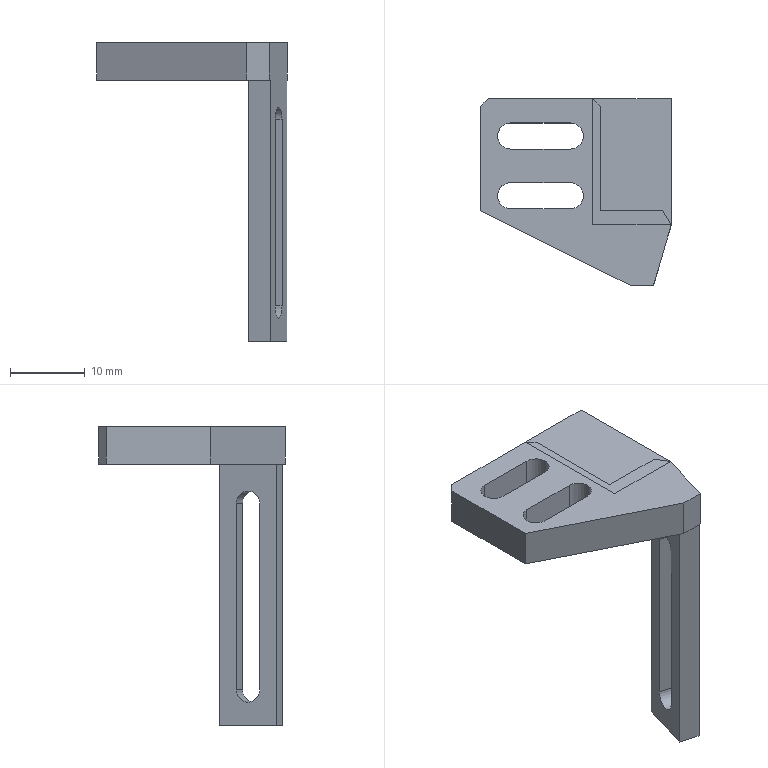NC program | NX | posted with a generic post | part box 25.523 x 25 x 40 mm
Whole program:
N10 G17 G21 G94 G90
(ZLEVEL_PROFILE_1_1 , TOOL : D4R0.5)
N12 T07 M6
N14 G54
N16 G17 G0 G90 X2.815 Y14.477 B0. C0. S7500 M3
N18 G43 Z30. H7
N20 Z0.948
N22 G94 G1 Z-0.052 F1000.
N24 X2.518 Y14.992
N26 G3 X2.172 Y15.192 R0.4
N28 G1 X-7.172 F2500.
N30 Y15.149 Z-0.078
N32 Y15.107 Z-0.105
N34 X-5. Y15.106
N36 X0.
N38 X2.172 Y15.107
N40 Y15.063 Z-0.131
N42 Y15.022 Z-0.157
N44 X0. Y15.021
N46 X-5.
N48 X-7.172 Y15.022
N50 Y14.978 Z-0.183
N52 Y14.936 Z-0.209
N54 X-5.
N56 X0.
N58 X2.172
N60 Y14.893 Z-0.235
N62 Y14.851 Z-0.261
N64 X0. Y14.85
N66 X-5.
N68 X-7.172 Y14.851
N70 Y14.808 Z-0.287
N72 Y14.766 Z-0.314
N74 X-5. Y14.765
N76 X0.
N78 X2.172 Y14.766
N80 Y14.722 Z-0.34
N82 Y14.68 Z-0.366
N84 X0.
N86 X-5.
N88 X-7.172
N90 Y14.637 Z-0.392
N92 Y14.595 Z-0.418
N94 X-5.
N96 X0.
N98 X2.172
N100 Y14.552 Z-0.444
N102 Y14.51 Z-0.47
N104 X0. Y14.509
N106 X-5.
N108 X-7.172 Y14.51
N110 Y14.467 Z-0.496
N112 Y14.425 Z-0.522
N114 X-5. Y14.424
N116 X0.
N118 X2.172 Y14.425
N120 Y14.381 Z-0.549
N122 Y14.339 Z-0.575
N124 X0.
N126 X-5.
N128 X-7.172
N130 Y14.296 Z-0.601
N132 Y14.254 Z-0.627
N134 X-5. Y14.253
N136 X0.
N138 X2.172 Y14.254
N140 Y14.211 Z-0.653
N142 Y14.169 Z-0.679
N144 X0. Y14.168
N146 X-5.
N148 X-7.172 Y14.169
N150 Y14.126 Z-0.705
N152 Y14.084 Z-0.731
N154 X-5. Y14.083
N156 X0.
N158 X2.172 Y14.084
N160 Y14.04 Z-0.758
N162 Y13.998 Z-0.784
N164 X0.
N166 X-5.
N168 X-7.172
N170 Y13.955 Z-0.81
N172 Y13.913 Z-0.836
N174 X-5. Y13.912
N176 X0.
N178 X2.172 Y13.913
N180 Y13.87 Z-0.862
N182 Y13.828 Z-0.888
N184 X0. Y13.827
N186 X-5.
N188 X-7.172 Y13.828
N190 Y13.785 Z-0.914
N192 Y13.743 Z-0.94
N194 X-5. Y13.742
N196 X0.
N198 X2.172 Y13.743
N200 Y13.699 Z-0.967
N202 Y13.657 Z-0.993
N204 X0.
N206 X-5.
N208 X-7.172
N210 Y13.614 Z-1.019
N212 Y13.572 Z-1.045
N214 X-5. Y13.571
N216 X0.
N218 X2.172 Y13.572
N220 Y13.529 Z-1.071
N222 Y13.487 Z-1.097
N224 X0. Y13.486
N226 X-5.
N228 X-7.172 Y13.487
N230 Y13.443 Z-1.123
N232 Y13.402 Z-1.149
N234 X-5. Y13.401
N236 X0.
N238 X2.172 Y13.402
N240 Y13.358 Z-1.176
N242 Y13.316 Z-1.202
N244 X0.
N246 X-5.
N248 X-7.172
N250 Y13.273 Z-1.228
N252 Y13.231 Z-1.254
N254 X2.172
N256 Y13.188 Z-1.28
N258 Y13.146 Z-1.306
N260 X-7.172
N262 Y13.102 Z-1.332
N264 Y13.06 Z-1.358
N266 X2.172
N268 Y13.017 Z-1.385
N270 Y12.975 Z-1.411
N272 X-7.172
N274 Y12.932 Z-1.437
N276 Y12.89 Z-1.463
N278 X2.172
N280 Y12.847 Z-1.489
N282 Y12.805 Z-1.515
N284 X-7.172
N286 Y12.771 Z-1.535
N288 Y12.739 Z-1.555
N290 X2.172
N292 Y12.706 Z-1.575
N294 Y12.674 Z-1.595
N296 X-7.172
N298 Y12.641 Z-1.615
N300 Y12.609 Z-1.635
N302 X2.172
N304 Y12.576 Z-1.655
N306 Y12.544 Z-1.675
N308 X-7.172
N310 G3 X-7.518 Y12.344 R0.4
N312 G1 X-7.816 Y11.828
N314 Z-0.675
N316 G0 Z30.
N318 M5
N320 M2